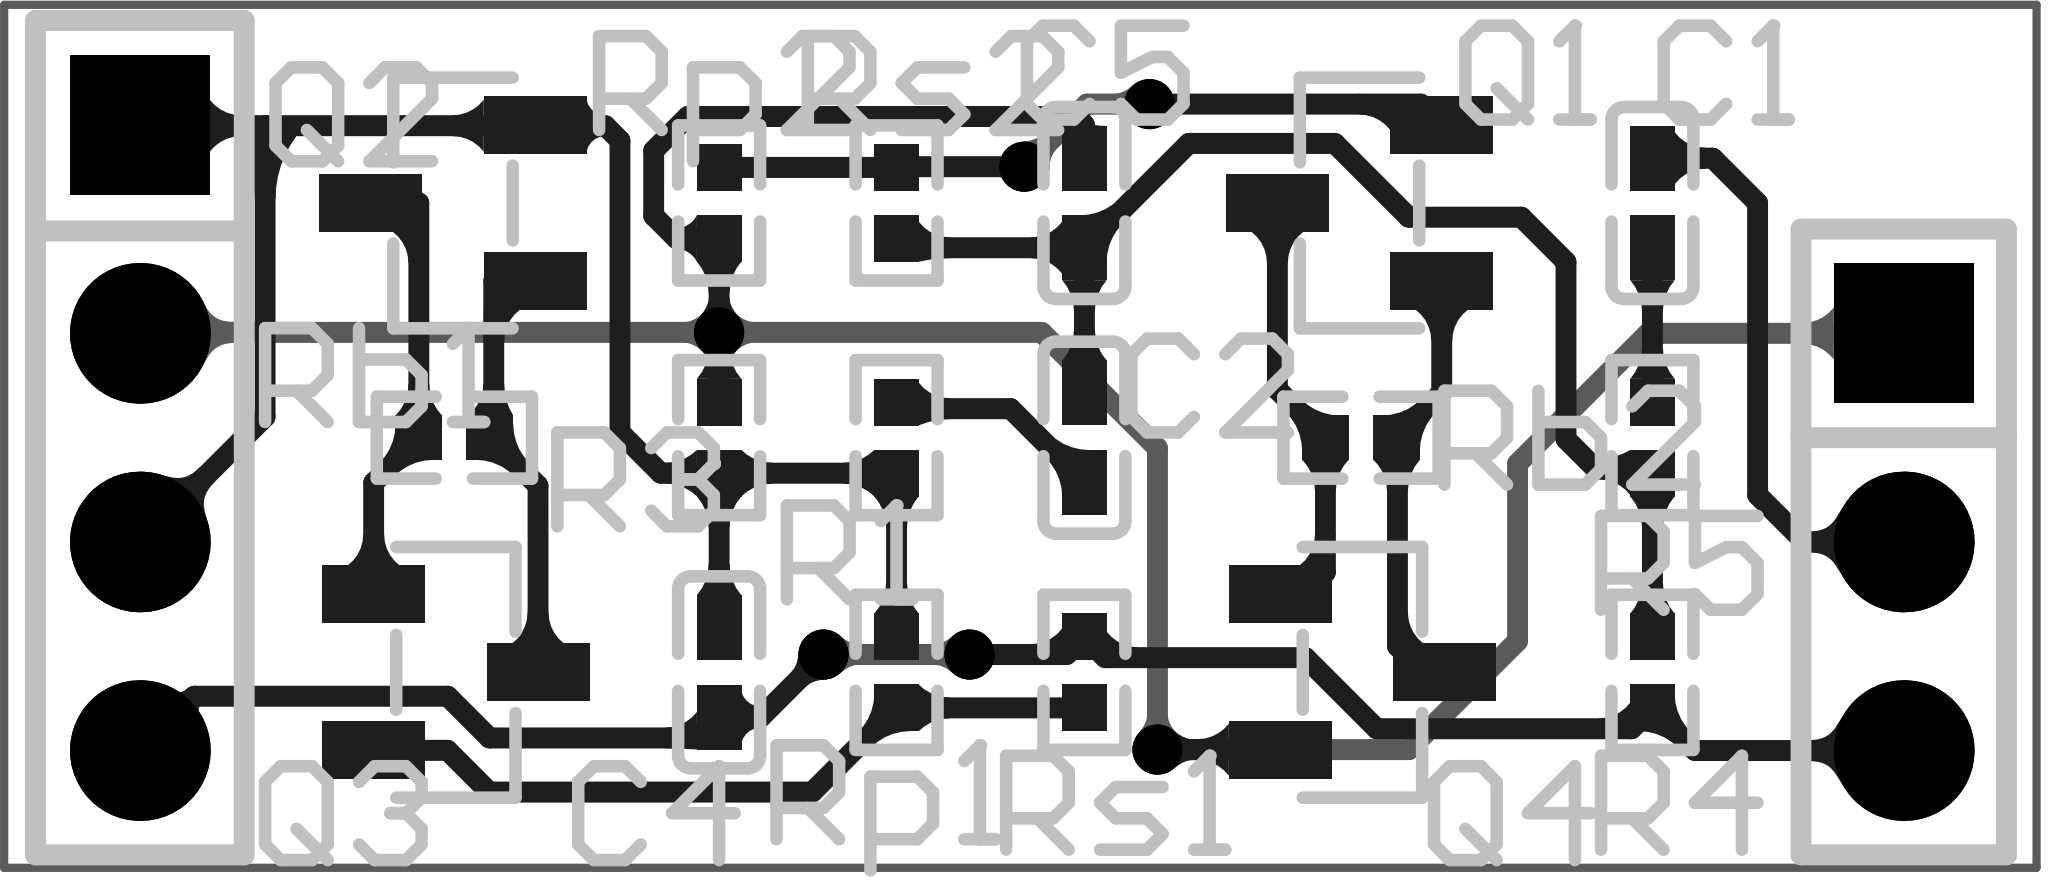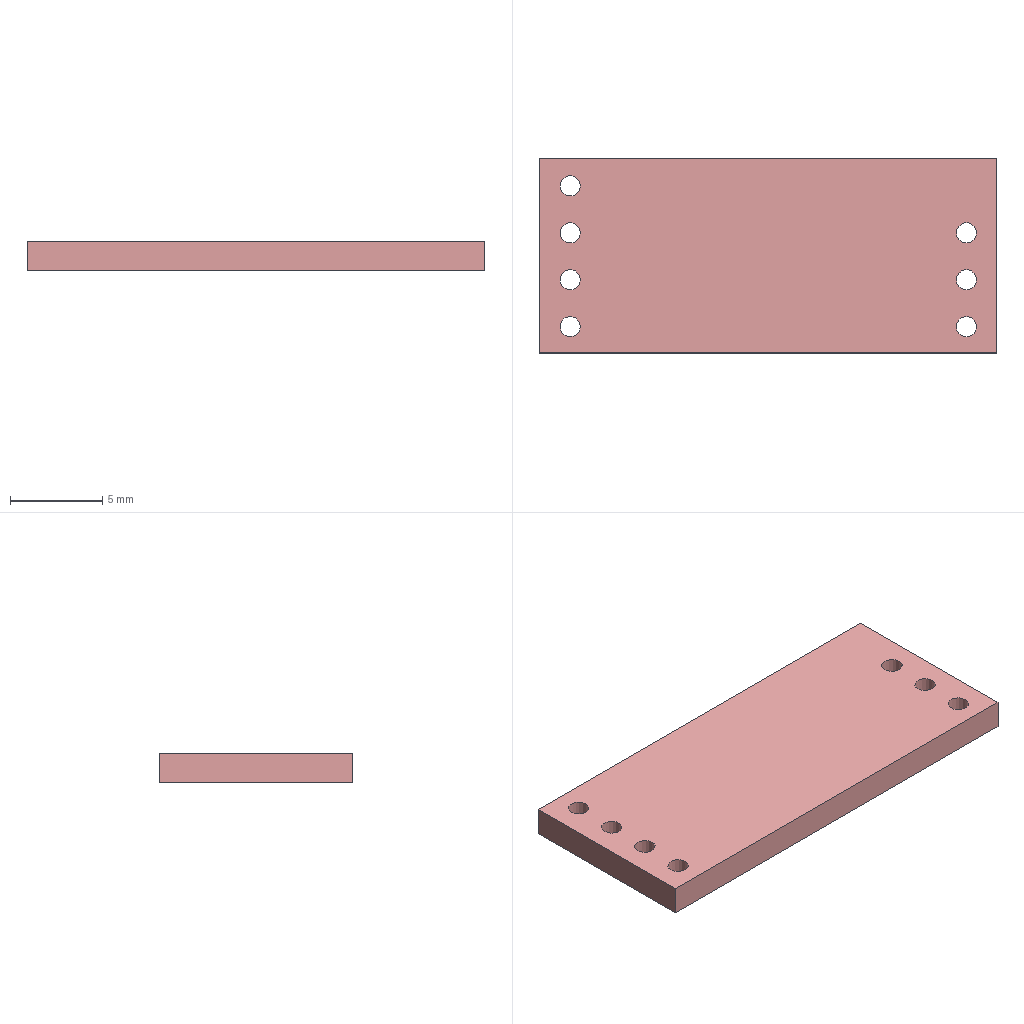Circuit board layout | Altium Designer | box 24.7 x 10.5 x 1.6 mm
Layer stack:
# Altium Designer layer stack of  (unit mm; dielectric type: 0 none, 1 core, 2 prepreg, 3 surface material)
index,name,kind,layer,copper_thickness_mm,dielectric_type,dielectric_thickness_mm,dielectric_material,dielectric_constant
0,Top Paste Mask Layer,other,,,,,,
1,Top Silkscreen Layer,other,,,,,,
2,Top Solder Mask Layer,dielectric,,,3,0.01,,3.3
3,Top Layer,copper,Top Layer,0.035,,,,
4,Dielectric1,dielectric,,,3,1.51,FR4,4.5
5,Bottom Layer,copper,Bottom Layer,0.035,,,,
6,Bottom Solder Mask Layer,dielectric,,,3,0.01,,3.3
7,Bottom Silkscreen Layer,other,,,,,,
8,Bottom Paste Mask Layer,other,,,,,,
# drill layer pairs: low layer,high layer
drill_pair,Top Layer,Bottom Layer
Part placement:
Designator,Comment,Layer,Footprint,Center-X(mm),Center-Y(mm),Rotation
C4,0.1uF,TopLayer,C0402,84.9,78.58,90
C5,0.1uF,TopLayer,C0402,89.344,84.295,90
C2,0.1uF,TopLayer,C0402,89.344,81.438,270
C1,0.1uF,TopLayer,C0402,96.256,84.295,270
H4,,TopLayer,HDR-TH_3P-P2.54-V-M,99.314,80.168,270
Q3,MMBT3906,TopLayer,SOT-23-3_L2.9-W1.3-P1.90-LS2.4-BR,81.696,78.58,180
Q2,MMBT3904,TopLayer,SOT-23-3_L2.9-W1.3-P1.90-LS2.4-BR,81.661,84.295,0
Q1,MMBT3906,TopLayer,SOT-23-3_L2.9-W1.3-P1.90-LS2.4-BR,92.692,84.295,0
Q4,MMBT3904,TopLayer,SOT-23-3_L2.9-W1.3-P1.90-LS2.4-BR,92.728,78.58,180
R3,2.2K,TopLayer,R0402,84.9,81.438,90
R4,2.2K,TopLayer,R0402,96.256,78.58,90
Rb1,1K,TopLayer,R0402,81.678,81.438,180
R1,1,TopLayer,R0402,87.058,81.438,270
Rb2,1K,TopLayer,R0402,92.71,81.438,0
R5,1,TopLayer,R0402,96.256,81.438,270
Rp1,200K,TopLayer,R0402,87.058,78.58,90
Rp2,200K,TopLayer,R0402,84.9,84.295,270
Rs1,200,TopLayer,R0402,89.344,78.58,90
Rs2,200,TopLayer,R0402,87.058,84.295,270
H3,,TopLayer,HDR-TH_4P-P2.54-V-M,77.851,81.438,270
Pad and via stacks:
# Altium Designer via and pad stacks of  (unit mm). Each distinct definition once, with the count of objects using it.
# via: kind,start_layer,end_layer,hole_mm,diameter_mm,mode(0 simple;1 top-mid-bottom;2 full stack),diameter_per_layer,count,example_net
# pad: kind,layer,hole_mm,hole_type(0 round;1 square;2 slot),plating,top_size,top_shape(1 round;2 rect;3 octagon;9 rounded rect),mid_size,bottom_size,mode,footprint,size_per_layer,count,example
pad,Top Layer,0,0,plated,0.7901x0.54,2,0.7901x0.54,0.7901x0.54,0,C0402,,8,C4.2
pad,Top Layer,0,0,plated,1.25x0.7,2,1.25x0.7,1.25x0.7,0,SOT-23-3_L2.9-W1.3-P1.90-LS2.4-BR,,12,Q3.1
pad,Top Layer,0,0,plated,0.5657x0.54,2,0.5657x0.54,0.5657x0.54,0,R0402,,20,R3.2
pad,Multi-Layer,1.1,0,plated,1.7x1.7,2,1.7x1.7,1.7x1.7,0,HDR-TH_3P-P2.54-V-M,,1,H4.1
pad,Multi-Layer,1.1,0,plated,1.7x1.7,1,1.7x1.7,1.7x1.7,0,HDR-TH_3P-P2.54-V-M,,2,H4.2
pad,Multi-Layer,1.1,0,plated,1.7x1.7,2,1.7x1.7,1.7x1.7,0,HDR-TH_4P-P2.54-V-M,,1,H3.1
pad,Multi-Layer,1.1,0,plated,1.7x1.7,1,1.7x1.7,1.7x1.7,0,HDR-TH_4P-P2.54-V-M,,3,H3.2
via,Top Layer,Bottom Layer,0.3048,0.61,0,,6,$1N1162